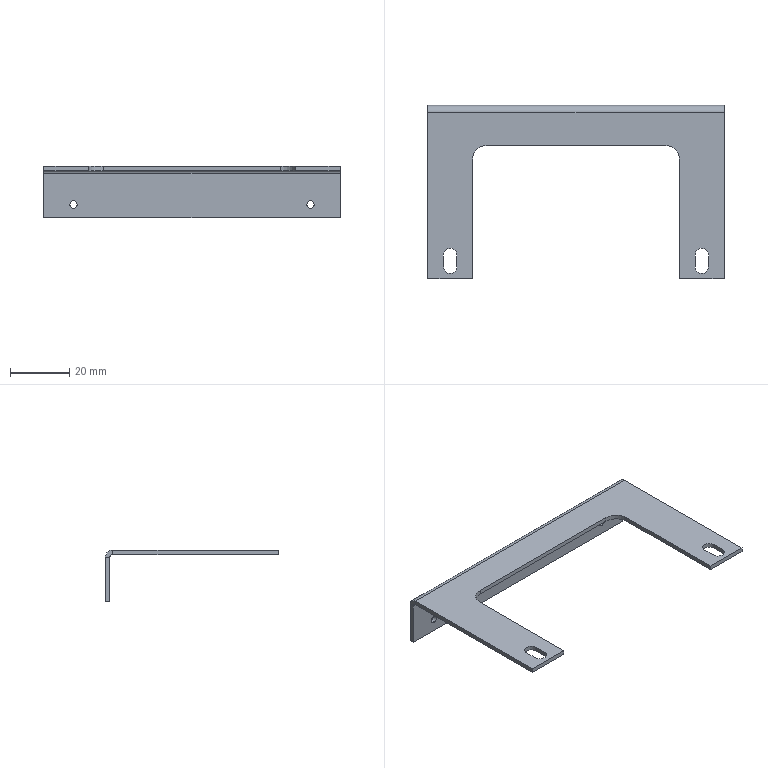Part | SolidWorks | features HoleWzd 2, Cut 1, FlatPattern 1, SMBaseFlange 1, SheetMetal 1 | 1 solid | 32 faces | box 100 x 58.5 x 17.5 mm | volume 6237 mm3 | plane 20 | cylinder 12 | commonest cylinder face diameters 2.5 x4 4.5 x4 10 x2 2 x1 5 x1
STEP:
#1=CARTESIAN_POINT('',(90.,58.5,-10.25));
#2=VERTEX_POINT('',#1);
#3=CARTESIAN_POINT('',(90.,58.5,-12.75));
#4=VERTEX_POINT('',#3);
#5=CARTESIAN_POINT('',(90.,58.5,-11.5));
#6=DIRECTION('',(0.,-1.,0.));
#7=DIRECTION('',(0.,0.,-1.));
#8=AXIS2_PLACEMENT_3D('',#5,#6,#7);
#9=CIRCLE('',#8,1.25);
#10=EDGE_CURVE('',#2,#4,#9,.T.);
#11=ORIENTED_EDGE('',*,*,#10,.F.);
#12=CARTESIAN_POINT('',(90.,57.,-10.25));
#13=VERTEX_POINT('',#12);
#14=CARTESIAN_POINT('',(90.,57.,-10.25));
#15=DIRECTION('',(0.,-1.,0.));
#16=VECTOR('',#15,1000.);
#17=LINE('',#14,#16);
#18=EDGE_CURVE('',#2,#13,#17,.T.);
#19=ORIENTED_EDGE('',*,*,#18,.T.);
#20=CARTESIAN_POINT('',(90.,57.,-12.75));
#21=VERTEX_POINT('',#20);
#22=CARTESIAN_POINT('',(90.,57.,-11.5));
#23=DIRECTION('',(0.,-1.,0.));
#24=DIRECTION('',(0.,0.,-1.));
#25=AXIS2_PLACEMENT_3D('',#22,#23,#24);
#26=CIRCLE('',#25,1.25);
#27=EDGE_CURVE('',#13,#21,#26,.T.);
#28=ORIENTED_EDGE('',*,*,#27,.T.);
#29=CARTESIAN_POINT('',(90.,57.,-12.75));
#30=DIRECTION('',(0.,-1.,0.));
#31=VECTOR('',#30,1000.);
#32=LINE('',#29,#31);
#33=EDGE_CURVE('',#4,#21,#32,.T.);
#34=ORIENTED_EDGE('',*,*,#33,.F.);
#35=EDGE_LOOP('',(#11,#19,#28,#34));
#36=FACE_OUTER_BOUND('',#35,.T.);
#37=CARTESIAN_POINT('',(90.,57.,-11.5));
#38=DIRECTION('',(0.,-1.,0.));
#39=DIRECTION('',(0.,0.,-1.));
#40=AXIS2_PLACEMENT_3D('',#37,#38,#39);
#41=CYLINDRICAL_SURFACE('',#40,1.25);
#42=ADVANCED_FACE('',(#36),#41,.F.);
#43=CARTESIAN_POINT('',(10.,58.5,-10.25));
#44=VERTEX_POINT('',#43);
#45=CARTESIAN_POINT('',(10.,58.5,-12.75));
#46=VERTEX_POINT('',#45);
#47=CARTESIAN_POINT('',(10.,58.5,-11.5));
#48=DIRECTION('',(0.,-1.,0.));
#49=DIRECTION('',(0.,0.,-1.));
#50=AXIS2_PLACEMENT_3D('',#47,#48,#49);
#51=CIRCLE('',#50,1.25);
#52=EDGE_CURVE('',#44,#46,#51,.T.);
#53=ORIENTED_EDGE('',*,*,#52,.F.);
#54=CARTESIAN_POINT('',(10.,57.,-10.25));
#55=VERTEX_POINT('',#54);
#56=CARTESIAN_POINT('',(10.,57.,-10.25));
#57=DIRECTION('',(0.,-1.,0.));
#58=VECTOR('',#57,1000.);
#59=LINE('',#56,#58);
#60=EDGE_CURVE('',#44,#55,#59,.T.);
#61=ORIENTED_EDGE('',*,*,#60,.T.);
#62=CARTESIAN_POINT('',(10.,57.,-12.75));
#63=VERTEX_POINT('',#62);
#64=CARTESIAN_POINT('',(10.,57.,-11.5));
#65=DIRECTION('',(0.,-1.,0.));
#66=DIRECTION('',(0.,0.,-1.));
#67=AXIS2_PLACEMENT_3D('',#64,#65,#66);
#68=CIRCLE('',#67,1.25);
#69=EDGE_CURVE('',#55,#63,#68,.T.);
#70=ORIENTED_EDGE('',*,*,#69,.T.);
#71=CARTESIAN_POINT('',(10.,57.,-12.75));
#72=DIRECTION('',(0.,-1.,0.));
#73=VECTOR('',#72,1000.);
#74=LINE('',#71,#73);
#75=EDGE_CURVE('',#46,#63,#74,.T.);
#76=ORIENTED_EDGE('',*,*,#75,.F.);
#77=EDGE_LOOP('',(#53,#61,#70,#76));
#78=FACE_OUTER_BOUND('',#77,.T.);
#79=CARTESIAN_POINT('',(10.,57.,-11.5));
#80=DIRECTION('',(0.,-1.,0.));
#81=DIRECTION('',(0.,0.,-1.));
#82=AXIS2_PLACEMENT_3D('',#79,#80,#81);
#83=CYLINDRICAL_SURFACE('',#82,1.25);
#84=ADVANCED_FACE('',(#78),#83,.F.);
#85=CARTESIAN_POINT('',(15.,0.,0.));
#86=VERTEX_POINT('',#85);
#87=CARTESIAN_POINT('',(15.,0.,1.5));
#88=VERTEX_POINT('',#87);
#89=CARTESIAN_POINT('',(15.,0.,-16.));
#90=DIRECTION('',(0.,0.,1.));
#91=VECTOR('',#90,1000.);
#92=LINE('',#89,#91);
#93=EDGE_CURVE('',#86,#88,#92,.T.);
#94=ORIENTED_EDGE('',*,*,#93,.T.);
#95=CARTESIAN_POINT('',(0.,0.,1.5));
#96=VERTEX_POINT('',#95);
#97=CARTESIAN_POINT('',(100.,0.,1.5));
#98=DIRECTION('',(-1.,0.,0.));
#99=VECTOR('',#98,1000.);
#100=LINE('',#97,#99);
#101=EDGE_CURVE('',#88,#96,#100,.T.);
#102=ORIENTED_EDGE('',*,*,#101,.T.);
#103=CARTESIAN_POINT('',(0.,0.,0.));
#104=VERTEX_POINT('',#103);
#105=CARTESIAN_POINT('',(0.,0.,0.));
#106=DIRECTION('',(0.,0.,1.));
#107=VECTOR('',#106,1000.);
#108=LINE('',#105,#107);
#109=EDGE_CURVE('',#104,#96,#108,.T.);
#110=ORIENTED_EDGE('',*,*,#109,.F.);
#111=CARTESIAN_POINT('',(100.,0.,0.));
#112=DIRECTION('',(-1.,0.,0.));
#113=VECTOR('',#112,1000.);
#114=LINE('',#111,#113);
#115=EDGE_CURVE('',#86,#104,#114,.T.);
#116=ORIENTED_EDGE('',*,*,#115,.F.);
#117=EDGE_LOOP('',(#94,#102,#110,#116));
#118=FACE_OUTER_BOUND('',#117,.T.);
#119=CARTESIAN_POINT('',(100.,0.,0.));
#120=DIRECTION('',(0.,-1.,0.));
#121=DIRECTION('',(0.,0.,-1.));
#122=AXIS2_PLACEMENT_3D('',#119,#120,#121);
#123=PLANE('',#122);
#124=ADVANCED_FACE('',(#118),#123,.T.);
#125=CARTESIAN_POINT('',(100.,56.,0.));
#126=VERTEX_POINT('',#125);
#127=CARTESIAN_POINT('',(100.,56.,1.5));
#128=VERTEX_POINT('',#127);
#129=CARTESIAN_POINT('',(100.,56.,0.));
#130=DIRECTION('',(0.,0.,1.));
#131=VECTOR('',#130,1000.);
#132=LINE('',#129,#131);
#133=EDGE_CURVE('',#126,#128,#132,.T.);
#134=ORIENTED_EDGE('',*,*,#133,.F.);
#135=CARTESIAN_POINT('',(100.,57.,-1.));
#136=VERTEX_POINT('',#135);
#137=CARTESIAN_POINT('',(100.,56.,-1.));
#138=DIRECTION('',(1.,0.,0.));
#139=DIRECTION('',(0.,0.,-1.));
#140=AXIS2_PLACEMENT_3D('',#137,#138,#139);
#141=CIRCLE('',#140,1.);
#142=EDGE_CURVE('',#136,#126,#141,.T.);
#143=ORIENTED_EDGE('',*,*,#142,.F.);
#144=CARTESIAN_POINT('',(100.,58.5,-1.));
#145=VERTEX_POINT('',#144);
#146=CARTESIAN_POINT('',(100.,58.5,-1.));
#147=DIRECTION('',(0.,-1.,0.));
#148=VECTOR('',#147,1000.);
#149=LINE('',#146,#148);
#150=EDGE_CURVE('',#145,#136,#149,.T.);
#151=ORIENTED_EDGE('',*,*,#150,.F.);
#152=CARTESIAN_POINT('',(100.,56.,-1.));
#153=DIRECTION('',(1.,0.,0.));
#154=DIRECTION('',(0.,0.,-1.));
#155=AXIS2_PLACEMENT_3D('',#152,#153,#154);
#156=CIRCLE('',#155,2.5);
#157=EDGE_CURVE('',#145,#128,#156,.T.);
#158=ORIENTED_EDGE('',*,*,#157,.T.);
#159=EDGE_LOOP('',(#134,#143,#151,#158));
#160=FACE_OUTER_BOUND('',#159,.T.);
#161=CARTESIAN_POINT('',(100.,56.,0.));
#162=DIRECTION('',(1.,0.,0.));
#163=DIRECTION('',(0.,0.,-1.));
#164=AXIS2_PLACEMENT_3D('',#161,#162,#163);
#165=PLANE('',#164);
#166=ADVANCED_FACE('',(#160),#165,.T.);
#167=CARTESIAN_POINT('',(100.,0.,0.));
#168=VERTEX_POINT('',#167);
#169=CARTESIAN_POINT('',(100.,0.,0.));
#170=DIRECTION('',(0.,-1.,0.));
#171=VECTOR('',#170,1000.);
#172=LINE('',#169,#171);
#173=EDGE_CURVE('',#126,#168,#172,.T.);
#174=ORIENTED_EDGE('',*,*,#173,.F.);
#175=ORIENTED_EDGE('',*,*,#133,.T.);
#176=CARTESIAN_POINT('',(100.,0.,1.5));
#177=VERTEX_POINT('',#176);
#178=CARTESIAN_POINT('',(100.,0.,1.5));
#179=DIRECTION('',(0.,-1.,0.));
#180=VECTOR('',#179,1000.);
#181=LINE('',#178,#180);
#182=EDGE_CURVE('',#128,#177,#181,.T.);
#183=ORIENTED_EDGE('',*,*,#182,.T.);
#184=CARTESIAN_POINT('',(100.,0.,0.));
#185=DIRECTION('',(0.,0.,1.));
#186=VECTOR('',#185,1000.);
#187=LINE('',#184,#186);
#188=EDGE_CURVE('',#168,#177,#187,.T.);
#189=ORIENTED_EDGE('',*,*,#188,.F.);
#190=EDGE_LOOP('',(#174,#175,#183,#189));
#191=FACE_OUTER_BOUND('',#190,.T.);
#192=CARTESIAN_POINT('',(100.,58.5,-1.));
#193=DIRECTION('',(1.,0.,0.));
#194=DIRECTION('',(0.,0.,-1.));
#195=AXIS2_PLACEMENT_3D('',#192,#193,#194);
#196=PLANE('',#195);
#197=ADVANCED_FACE('',(#191),#196,.T.);
#198=CARTESIAN_POINT('',(0.,57.,-1.));
#199=VERTEX_POINT('',#198);
#200=CARTESIAN_POINT('',(0.,58.5,-1.));
#201=VERTEX_POINT('',#200);
#202=CARTESIAN_POINT('',(0.,57.,-1.));
#203=DIRECTION('',(0.,1.,0.));
#204=VECTOR('',#203,1000.);
#205=LINE('',#202,#204);
#206=EDGE_CURVE('',#199,#201,#205,.T.);
#207=ORIENTED_EDGE('',*,*,#206,.F.);
#208=CARTESIAN_POINT('',(0.,56.,0.));
#209=VERTEX_POINT('',#208);
#210=CARTESIAN_POINT('',(0.,56.,-1.));
#211=DIRECTION('',(1.,0.,0.));
#212=DIRECTION('',(0.,0.,-1.));
#213=AXIS2_PLACEMENT_3D('',#210,#211,#212);
#214=CIRCLE('',#213,1.);
#215=EDGE_CURVE('',#199,#209,#214,.T.);
#216=ORIENTED_EDGE('',*,*,#215,.T.);
#217=CARTESIAN_POINT('',(0.,56.,1.5));
#218=VERTEX_POINT('',#217);
#219=CARTESIAN_POINT('',(0.,56.,1.5));
#220=DIRECTION('',(0.,0.,-1.));
#221=VECTOR('',#220,1000.);
#222=LINE('',#219,#221);
#223=EDGE_CURVE('',#218,#209,#222,.T.);
#224=ORIENTED_EDGE('',*,*,#223,.F.);
#225=CARTESIAN_POINT('',(0.,56.,-1.));
#226=DIRECTION('',(1.,0.,0.));
#227=DIRECTION('',(0.,0.,-1.));
#228=AXIS2_PLACEMENT_3D('',#225,#226,#227);
#229=CIRCLE('',#228,2.5);
#230=EDGE_CURVE('',#201,#218,#229,.T.);
#231=ORIENTED_EDGE('',*,*,#230,.F.);
#232=EDGE_LOOP('',(#207,#216,#224,#231));
#233=FACE_OUTER_BOUND('',#232,.T.);
#234=CARTESIAN_POINT('',(0.,57.,-1.));
#235=DIRECTION('',(-1.,0.,0.));
#236=DIRECTION('',(0.,0.,1.));
#237=AXIS2_PLACEMENT_3D('',#234,#235,#236);
#238=PLANE('',#237);
#239=ADVANCED_FACE('',(#233),#238,.T.);
#240=CARTESIAN_POINT('',(0.,57.,-16.));
#241=VERTEX_POINT('',#240);
#242=CARTESIAN_POINT('',(0.,57.,0.));
#243=DIRECTION('',(0.,0.,1.));
#244=VECTOR('',#243,1000.);
#245=LINE('',#242,#244);
#246=EDGE_CURVE('',#241,#199,#245,.T.);
#247=ORIENTED_EDGE('',*,*,#246,.T.);
#248=ORIENTED_EDGE('',*,*,#206,.T.);
#249=CARTESIAN_POINT('',(0.,58.5,-16.));
#250=VERTEX_POINT('',#249);
#251=CARTESIAN_POINT('',(0.,58.5,0.));
#252=DIRECTION('',(0.,0.,1.));
#253=VECTOR('',#252,1000.);
#254=LINE('',#251,#253);
#255=EDGE_CURVE('',#250,#201,#254,.T.);
#256=ORIENTED_EDGE('',*,*,#255,.F.);
#257=CARTESIAN_POINT('',(0.,58.5,-16.));
#258=DIRECTION('',(0.,-1.,0.));
#259=VECTOR('',#258,1000.);
#260=LINE('',#257,#259);
#261=EDGE_CURVE('',#250,#241,#260,.T.);
#262=ORIENTED_EDGE('',*,*,#261,.T.);
#263=EDGE_LOOP('',(#247,#248,#256,#262));
#264=FACE_OUTER_BOUND('',#263,.T.);
#265=CARTESIAN_POINT('',(0.,56.,1.5));
#266=DIRECTION('',(-1.,0.,0.));
#267=DIRECTION('',(0.,0.,1.));
#268=AXIS2_PLACEMENT_3D('',#265,#266,#267);
#269=PLANE('',#268);
#270=ADVANCED_FACE('',(#264),#269,.T.);
#271=CARTESIAN_POINT('',(94.75,8.,1.5));
#272=VERTEX_POINT('',#271);
#273=CARTESIAN_POINT('',(90.25,8.,1.5));
#274=VERTEX_POINT('',#273);
#275=CARTESIAN_POINT('',(92.5,8.,1.5));
#276=DIRECTION('',(0.,0.,1.));
#277=DIRECTION('',(1.,0.,0.));
#278=AXIS2_PLACEMENT_3D('',#275,#276,#277);
#279=CIRCLE('',#278,2.25);
#280=EDGE_CURVE('',#272,#274,#279,.T.);
#281=ORIENTED_EDGE('',*,*,#280,.F.);
#282=CARTESIAN_POINT('',(94.75,4.,1.5));
#283=VERTEX_POINT('',#282);
#284=CARTESIAN_POINT('',(94.75,4.,1.5));
#285=DIRECTION('',(0.,1.,0.));
#286=VECTOR('',#285,1000.);
#287=LINE('',#284,#286);
#288=EDGE_CURVE('',#283,#272,#287,.T.);
#289=ORIENTED_EDGE('',*,*,#288,.F.);
#290=CARTESIAN_POINT('',(90.25,4.,1.5));
#291=VERTEX_POINT('',#290);
#292=CARTESIAN_POINT('',(92.5,4.,1.5));
#293=DIRECTION('',(0.,0.,1.));
#294=DIRECTION('',(1.,0.,0.));
#295=AXIS2_PLACEMENT_3D('',#292,#293,#294);
#296=CIRCLE('',#295,2.25);
#297=EDGE_CURVE('',#291,#283,#296,.T.);
#298=ORIENTED_EDGE('',*,*,#297,.F.);
#299=CARTESIAN_POINT('',(90.25,4.,1.5));
#300=DIRECTION('',(0.,1.,0.));
#301=VECTOR('',#300,1000.);
#302=LINE('',#299,#301);
#303=EDGE_CURVE('',#291,#274,#302,.T.);
#304=ORIENTED_EDGE('',*,*,#303,.T.);
#305=EDGE_LOOP('',(#281,#289,#298,#304));
#306=FACE_BOUND('',#305,.T.);
#307=CARTESIAN_POINT('',(9.75,4.,1.5));
#308=VERTEX_POINT('',#307);
#309=CARTESIAN_POINT('',(9.75,8.,1.5));
#310=VERTEX_POINT('',#309);
#311=CARTESIAN_POINT('',(9.75,4.,1.5));
#312=DIRECTION('',(0.,1.,0.));
#313=VECTOR('',#312,1000.);
#314=LINE('',#311,#313);
#315=EDGE_CURVE('',#308,#310,#314,.T.);
#316=ORIENTED_EDGE('',*,*,#315,.F.);
#317=CARTESIAN_POINT('',(5.25,4.,1.5));
#318=VERTEX_POINT('',#317);
#319=CARTESIAN_POINT('',(7.5,4.,1.5));
#320=DIRECTION('',(0.,0.,1.));
#321=DIRECTION('',(1.,0.,0.));
#322=AXIS2_PLACEMENT_3D('',#319,#320,#321);
#323=CIRCLE('',#322,2.25);
#324=EDGE_CURVE('',#318,#308,#323,.T.);
#325=ORIENTED_EDGE('',*,*,#324,.F.);
#326=CARTESIAN_POINT('',(5.25,8.,1.5));
#327=VERTEX_POINT('',#326);
#328=CARTESIAN_POINT('',(5.25,4.,1.5));
#329=DIRECTION('',(0.,1.,0.));
#330=VECTOR('',#329,1000.);
#331=LINE('',#328,#330);
#332=EDGE_CURVE('',#318,#327,#331,.T.);
#333=ORIENTED_EDGE('',*,*,#332,.T.);
#334=CARTESIAN_POINT('',(7.5,8.,1.5));
#335=DIRECTION('',(0.,0.,1.));
#336=DIRECTION('',(1.,0.,0.));
#337=AXIS2_PLACEMENT_3D('',#334,#335,#336);
#338=CIRCLE('',#337,2.25);
#339=EDGE_CURVE('',#310,#327,#338,.T.);
#340=ORIENTED_EDGE('',*,*,#339,.F.);
#341=EDGE_LOOP('',(#316,#325,#333,#340));
#342=FACE_BOUND('',#341,.T.);
#343=ORIENTED_EDGE('',*,*,#101,.F.);
#344=CARTESIAN_POINT('',(15.,40.,1.5));
#345=VERTEX_POINT('',#344);
#346=CARTESIAN_POINT('',(15.,0.,1.5));
#347=DIRECTION('',(0.,-1.,0.));
#348=VECTOR('',#347,1000.);
#349=LINE('',#346,#348);
#350=EDGE_CURVE('',#345,#88,#349,.T.);
#351=ORIENTED_EDGE('',*,*,#350,.F.);
#352=CARTESIAN_POINT('',(20.,45.,1.5));
#353=VERTEX_POINT('',#352);
#354=CARTESIAN_POINT('',(20.,40.,1.5));
#355=DIRECTION('',(0.,0.,1.));
#356=DIRECTION('',(-1.,0.,0.));
#357=AXIS2_PLACEMENT_3D('',#354,#355,#356);
#358=CIRCLE('',#357,5.);
#359=EDGE_CURVE('',#353,#345,#358,.T.);
#360=ORIENTED_EDGE('',*,*,#359,.F.);
#361=CARTESIAN_POINT('',(80.,45.,1.5));
#362=VERTEX_POINT('',#361);
#363=CARTESIAN_POINT('',(20.,45.,1.5));
#364=DIRECTION('',(-1.,0.,0.));
#365=VECTOR('',#364,1000.);
#366=LINE('',#363,#365);
#367=EDGE_CURVE('',#362,#353,#366,.T.);
#368=ORIENTED_EDGE('',*,*,#367,.F.);
#369=CARTESIAN_POINT('',(85.,40.,1.5));
#370=VERTEX_POINT('',#369);
#371=CARTESIAN_POINT('',(80.,40.,1.5));
#372=DIRECTION('',(0.,0.,1.));
#373=DIRECTION('',(-1.,0.,0.));
#374=AXIS2_PLACEMENT_3D('',#371,#372,#373);
#375=CIRCLE('',#374,5.);
#376=EDGE_CURVE('',#370,#362,#375,.T.);
#377=ORIENTED_EDGE('',*,*,#376,.F.);
#378=CARTESIAN_POINT('',(85.,0.,1.5));
#379=VERTEX_POINT('',#378);
#380=CARTESIAN_POINT('',(85.,0.,1.5));
#381=DIRECTION('',(0.,1.,0.));
#382=VECTOR('',#381,1000.);
#383=LINE('',#380,#382);
#384=EDGE_CURVE('',#379,#370,#383,.T.);
#385=ORIENTED_EDGE('',*,*,#384,.F.);
#386=CARTESIAN_POINT('',(100.,0.,1.5));
#387=DIRECTION('',(-1.,0.,0.));
#388=VECTOR('',#387,1000.);
#389=LINE('',#386,#388);
#390=EDGE_CURVE('',#177,#379,#389,.T.);
#391=ORIENTED_EDGE('',*,*,#390,.F.);
#392=ORIENTED_EDGE('',*,*,#182,.F.);
#393=CARTESIAN_POINT('',(100.,56.,1.5));
#394=DIRECTION('',(-1.,0.,0.));
#395=VECTOR('',#394,1000.);
#396=LINE('',#393,#395);
#397=EDGE_CURVE('',#128,#218,#396,.T.);
#398=ORIENTED_EDGE('',*,*,#397,.T.);
#399=CARTESIAN_POINT('',(0.,0.,1.5));
#400=DIRECTION('',(0.,-1.,0.));
#401=VECTOR('',#400,1000.);
#402=LINE('',#399,#401);
#403=EDGE_CURVE('',#218,#96,#402,.T.);
#404=ORIENTED_EDGE('',*,*,#403,.T.);
#405=EDGE_LOOP('',(#343,#351,#360,#368,#377,#385,#391,#392,#398,#404));
#406=FACE_OUTER_BOUND('',#405,.T.);
#407=CARTESIAN_POINT('',(100.,0.,1.5));
#408=DIRECTION('',(0.,0.,-1.));
#409=DIRECTION('',(-1.,0.,0.));
#410=AXIS2_PLACEMENT_3D('',#407,#408,#409);
#411=PLANE('',#410);
#412=ADVANCED_FACE('',(#306,#342,#406),#411,.F.);
#413=CARTESIAN_POINT('',(85.,0.,0.));
#414=VERTEX_POINT('',#413);
#415=CARTESIAN_POINT('',(85.,0.,-16.));
#416=DIRECTION('',(0.,0.,1.));
#417=VECTOR('',#416,1000.);
#418=LINE('',#415,#417);
#419=EDGE_CURVE('',#414,#379,#418,.T.);
#420=ORIENTED_EDGE('',*,*,#419,.F.);
#421=CARTESIAN_POINT('',(100.,0.,0.));
#422=DIRECTION('',(-1.,0.,0.));
#423=VECTOR('',#422,1000.);
#424=LINE('',#421,#423);
#425=EDGE_CURVE('',#168,#414,#424,.T.);
#426=ORIENTED_EDGE('',*,*,#425,.F.);
#427=ORIENTED_EDGE('',*,*,#188,.T.);
#428=ORIENTED_EDGE('',*,*,#390,.T.);
#429=EDGE_LOOP('',(#420,#426,#427,#428));
#430=FACE_OUTER_BOUND('',#429,.T.);
#431=CARTESIAN_POINT('',(100.,0.,0.));
#432=DIRECTION('',(0.,-1.,0.));
#433=DIRECTION('',(0.,0.,-1.));
#434=AXIS2_PLACEMENT_3D('',#431,#432,#433);
#435=PLANE('',#434);
#436=ADVANCED_FACE('',(#430),#435,.T.);
#437=CARTESIAN_POINT('',(90.25,8.,0.));
#438=VERTEX_POINT('',#437);
#439=CARTESIAN_POINT('',(94.75,8.,0.));
#440=VERTEX_POINT('',#439);
#441=CARTESIAN_POINT('',(92.5,8.,0.));
#442=DIRECTION('',(0.,0.,-1.));
#443=DIRECTION('',(-1.,0.,0.));
#444=AXIS2_PLACEMENT_3D('',#441,#442,#443);
#445=CIRCLE('',#444,2.25);
#446=EDGE_CURVE('',#438,#440,#445,.T.);
#447=ORIENTED_EDGE('',*,*,#446,.F.);
#448=CARTESIAN_POINT('',(90.25,4.,0.));
#449=VERTEX_POINT('',#448);
#450=CARTESIAN_POINT('',(90.25,0.,0.));
#451=DIRECTION('',(0.,1.,0.));
#452=VECTOR('',#451,1000.);
#453=LINE('',#450,#452);
#454=EDGE_CURVE('',#449,#438,#453,.T.);
#455=ORIENTED_EDGE('',*,*,#454,.F.);
#456=CARTESIAN_POINT('',(94.75,4.,0.));
#457=VERTEX_POINT('',#456);
#458=CARTESIAN_POINT('',(92.5,4.,0.));
#459=DIRECTION('',(0.,0.,-1.));
#460=DIRECTION('',(-1.,0.,0.));
#461=AXIS2_PLACEMENT_3D('',#458,#459,#460);
#462=CIRCLE('',#461,2.25);
#463=EDGE_CURVE('',#457,#449,#462,.T.);
#464=ORIENTED_EDGE('',*,*,#463,.F.);
#465=CARTESIAN_POINT('',(94.75,0.,0.));
#466=DIRECTION('',(0.,-1.,0.));
#467=VECTOR('',#466,1000.);
#468=LINE('',#465,#467);
#469=EDGE_CURVE('',#440,#457,#468,.T.);
#470=ORIENTED_EDGE('',*,*,#469,.F.);
#471=EDGE_LOOP('',(#447,#455,#464,#470));
#472=FACE_BOUND('',#471,.T.);
#473=CARTESIAN_POINT('',(5.25,8.,0.));
#474=VERTEX_POINT('',#473);
#475=CARTESIAN_POINT('',(9.75,8.,0.));
#476=VERTEX_POINT('',#475);
#477=CARTESIAN_POINT('',(7.5,8.,0.));
#478=DIRECTION('',(0.,0.,-1.));
#479=DIRECTION('',(-1.,0.,0.));
#480=AXIS2_PLACEMENT_3D('',#477,#478,#479);
#481=CIRCLE('',#480,2.25);
#482=EDGE_CURVE('',#474,#476,#481,.T.);
#483=ORIENTED_EDGE('',*,*,#482,.F.);
#484=CARTESIAN_POINT('',(5.25,4.,0.));
#485=VERTEX_POINT('',#484);
#486=CARTESIAN_POINT('',(5.25,0.,0.));
#487=DIRECTION('',(0.,1.,0.));
#488=VECTOR('',#487,1000.);
#489=LINE('',#486,#488);
#490=EDGE_CURVE('',#485,#474,#489,.T.);
#491=ORIENTED_EDGE('',*,*,#490,.F.);
#492=CARTESIAN_POINT('',(9.75,4.,0.));
#493=VERTEX_POINT('',#492);
#494=CARTESIAN_POINT('',(7.5,4.,0.));
#495=DIRECTION('',(0.,0.,-1.));
#496=DIRECTION('',(-1.,0.,0.));
#497=AXIS2_PLACEMENT_3D('',#494,#495,#496);
#498=CIRCLE('',#497,2.25);
#499=EDGE_CURVE('',#493,#485,#498,.T.);
#500=ORIENTED_EDGE('',*,*,#499,.F.);
#501=CARTESIAN_POINT('',(9.75,0.,0.));
#502=DIRECTION('',(0.,-1.,0.));
#503=VECTOR('',#502,1000.);
#504=LINE('',#501,#503);
#505=EDGE_CURVE('',#476,#493,#504,.T.);
#506=ORIENTED_EDGE('',*,*,#505,.F.);
#507=EDGE_LOOP('',(#483,#491,#500,#506));
#508=FACE_BOUND('',#507,.T.);
#509=CARTESIAN_POINT('',(15.,40.,0.));
#510=VERTEX_POINT('',#509);
#511=CARTESIAN_POINT('',(15.,0.,0.));
#512=DIRECTION('',(0.,1.,0.));
#513=VECTOR('',#512,1000.);
#514=LINE('',#511,#513);
#515=EDGE_CURVE('',#86,#510,#514,.T.);
#516=ORIENTED_EDGE('',*,*,#515,.F.);
#517=ORIENTED_EDGE('',*,*,#115,.T.);
#518=CARTESIAN_POINT('',(0.,0.,0.));
#519=DIRECTION('',(0.,-1.,0.));
#520=VECTOR('',#519,1000.);
#521=LINE('',#518,#520);
#522=EDGE_CURVE('',#209,#104,#521,.T.);
#523=ORIENTED_EDGE('',*,*,#522,.F.);
#524=CARTESIAN_POINT('',(100.,56.,0.));
#525=DIRECTION('',(-1.,0.,0.));
#526=VECTOR('',#525,1000.);
#527=LINE('',#524,#526);
#528=EDGE_CURVE('',#126,#209,#527,.T.);
#529=ORIENTED_EDGE('',*,*,#528,.F.);
#530=ORIENTED_EDGE('',*,*,#173,.T.);
#531=ORIENTED_EDGE('',*,*,#425,.T.);
#532=CARTESIAN_POINT('',(85.,40.,0.));
#533=VERTEX_POINT('',#532);
#534=CARTESIAN_POINT('',(85.,0.,0.));
#535=DIRECTION('',(0.,-1.,0.));
#536=VECTOR('',#535,1000.);
#537=LINE('',#534,#536);
#538=EDGE_CURVE('',#533,#414,#537,.T.);
#539=ORIENTED_EDGE('',*,*,#538,.F.);
#540=CARTESIAN_POINT('',(80.,45.,0.));
#541=VERTEX_POINT('',#540);
#542=CARTESIAN_POINT('',(80.,40.,0.));
#543=DIRECTION('',(0.,0.,-1.));
#544=DIRECTION('',(-1.,0.,0.));
#545=AXIS2_PLACEMENT_3D('',#542,#543,#544);
#546=CIRCLE('',#545,5.);
#547=EDGE_CURVE('',#541,#533,#546,.T.);
#548=ORIENTED_EDGE('',*,*,#547,.F.);
#549=CARTESIAN_POINT('',(20.,45.,0.));
#550=VERTEX_POINT('',#549);
#551=CARTESIAN_POINT('',(100.,45.,0.));
#552=DIRECTION('',(1.,0.,0.));
#553=VECTOR('',#552,1000.);
#554=LINE('',#551,#553);
#555=EDGE_CURVE('',#550,#541,#554,.T.);
#556=ORIENTED_EDGE('',*,*,#555,.F.);
#557=CARTESIAN_POINT('',(20.,40.,0.));
#558=DIRECTION('',(0.,0.,-1.));
#559=DIRECTION('',(-1.,0.,0.));
#560=AXIS2_PLACEMENT_3D('',#557,#558,#559);
#561=CIRCLE('',#560,5.);
#562=EDGE_CURVE('',#510,#550,#561,.T.);
#563=ORIENTED_EDGE('',*,*,#562,.F.);
#564=EDGE_LOOP('',(#516,#517,#523,#529,#530,#531,#539,#548,#556,#563));
#565=FACE_OUTER_BOUND('',#564,.T.);
#566=CARTESIAN_POINT('',(100.,0.,0.));
#567=DIRECTION('',(0.,0.,-1.));
#568=DIRECTION('',(-1.,0.,0.));
#569=AXIS2_PLACEMENT_3D('',#566,#567,#568);
#570=PLANE('',#569);
#571=ADVANCED_FACE('',(#472,#508,#565),#570,.T.);
#572=ORIENTED_EDGE('',*,*,#215,.F.);
#573=CARTESIAN_POINT('',(100.,57.,-1.));
#574=DIRECTION('',(-1.,0.,0.));
#575=VECTOR('',#574,1000.);
#576=LINE('',#573,#575);
#577=EDGE_CURVE('',#136,#199,#576,.T.);
#578=ORIENTED_EDGE('',*,*,#577,.F.);
#579=ORIENTED_EDGE('',*,*,#142,.T.);
#580=ORIENTED_EDGE('',*,*,#528,.T.);
#581=EDGE_LOOP('',(#572,#578,#579,#580));
#582=FACE_OUTER_BOUND('',#581,.T.);
#583=CARTESIAN_POINT('',(100.,56.,-1.));
#584=DIRECTION('',(-1.,0.,0.));
#585=DIRECTION('',(0.,0.,1.));
#586=AXIS2_PLACEMENT_3D('',#583,#584,#585);
#587=CYLINDRICAL_SURFACE('',#586,1.);
#588=ADVANCED_FACE('',(#582),#587,.F.);
#589=CARTESIAN_POINT('',(90.,57.,-11.5));
#590=DIRECTION('',(0.,-1.,0.));
#591=DIRECTION('',(0.,0.,-1.));
#592=AXIS2_PLACEMENT_3D('',#589,#590,#591);
#593=CIRCLE('',#592,1.25);
#594=EDGE_CURVE('',#21,#13,#593,.T.);
#595=ORIENTED_EDGE('',*,*,#594,.F.);
#596=ORIENTED_EDGE('',*,*,#27,.F.);
#597=EDGE_LOOP('',(#595,#596));
#598=FACE_BOUND('',#597,.T.);
#599=CARTESIAN_POINT('',(10.,57.,-11.5));
#600=DIRECTION('',(0.,-1.,0.));
#601=DIRECTION('',(0.,0.,-1.));
#602=AXIS2_PLACEMENT_3D('',#599,#600,#601);
#603=CIRCLE('',#602,1.25);
#604=EDGE_CURVE('',#63,#55,#603,.T.);
#605=ORIENTED_EDGE('',*,*,#604,.F.);
#606=ORIENTED_EDGE('',*,*,#69,.F.);
#607=EDGE_LOOP('',(#605,#606));
#608=FACE_BOUND('',#607,.T.);
#609=ORIENTED_EDGE('',*,*,#246,.F.);
#610=CARTESIAN_POINT('',(100.,57.,-16.));
#611=VERTEX_POINT('',#610);
#612=CARTESIAN_POINT('',(100.,57.,-16.));
#613=DIRECTION('',(-1.,0.,0.));
#614=VECTOR('',#613,1000.);
#615=LINE('',#612,#614);
#616=EDGE_CURVE('',#611,#241,#615,.T.);
#617=ORIENTED_EDGE('',*,*,#616,.F.);
#618=CARTESIAN_POINT('',(100.,57.,0.));
#619=DIRECTION('',(0.,0.,1.));
#620=VECTOR('',#619,1000.);
#621=LINE('',#618,#620);
#622=EDGE_CURVE('',#611,#136,#621,.T.);
#623=ORIENTED_EDGE('',*,*,#622,.T.);
#624=ORIENTED_EDGE('',*,*,#577,.T.);
#625=EDGE_LOOP('',(#609,#617,#623,#624));
#626=FACE_OUTER_BOUND('',#625,.T.);
#627=CARTESIAN_POINT('',(100.,57.,0.));
#628=DIRECTION('',(0.,-1.,0.));
#629=DIRECTION('',(0.,0.,-1.));
#630=AXIS2_PLACEMENT_3D('',#627,#628,#629);
#631=PLANE('',#630);
#632=ADVANCED_FACE('',(#598,#608,#626),#631,.T.);
#633=ORIENTED_EDGE('',*,*,#261,.F.);
#634=CARTESIAN_POINT('',(100.,58.5,-16.));
#635=VERTEX_POINT('',#634);
#636=CARTESIAN_POINT('',(100.,58.5,-16.));
#637=DIRECTION('',(-1.,0.,0.));
#638=VECTOR('',#637,1000.);
#639=LINE('',#636,#638);
#640=EDGE_CURVE('',#635,#250,#639,.T.);
#641=ORIENTED_EDGE('',*,*,#640,.F.);
#642=CARTESIAN_POINT('',(100.,58.5,-16.));
#643=DIRECTION('',(0.,-1.,0.));
#644=VECTOR('',#643,1000.);
#645=LINE('',#642,#644);
#646=EDGE_CURVE('',#635,#611,#645,.T.);
#647=ORIENTED_EDGE('',*,*,#646,.T.);
#648=ORIENTED_EDGE('',*,*,#616,.T.);
#649=EDGE_LOOP('',(#633,#641,#647,#648));
#650=FACE_OUTER_BOUND('',#649,.T.);
#651=CARTESIAN_POINT('',(100.,58.5,-16.));
#652=DIRECTION('',(0.,0.,-1.));
#653=DIRECTION('',(-1.,0.,0.));
#654=AXIS2_PLACEMENT_3D('',#651,#652,#653);
#655=PLANE('',#654);
#656=ADVANCED_FACE('',(#650),#655,.T.);
#657=CARTESIAN_POINT('',(90.,58.5,-11.5));
#658=DIRECTION('',(0.,-1.,0.));
#659=DIRECTION('',(0.,0.,-1.));
#660=AXIS2_PLACEMENT_3D('',#657,#658,#659);
#661=CIRCLE('',#660,1.25);
#662=EDGE_CURVE('',#4,#2,#661,.T.);
#663=ORIENTED_EDGE('',*,*,#662,.T.);
#664=ORIENTED_EDGE('',*,*,#10,.T.);
#665=EDGE_LOOP('',(#663,#664));
#666=FACE_BOUND('',#665,.T.);
#667=CARTESIAN_POINT('',(10.,58.5,-11.5));
#668=DIRECTION('',(0.,-1.,0.));
#669=DIRECTION('',(0.,0.,-1.));
#670=AXIS2_PLACEMENT_3D('',#667,#668,#669);
#671=CIRCLE('',#670,1.25);
#672=EDGE_CURVE('',#46,#44,#671,.T.);
#673=ORIENTED_EDGE('',*,*,#672,.T.);
#674=ORIENTED_EDGE('',*,*,#52,.T.);
#675=EDGE_LOOP('',(#673,#674));
#676=FACE_BOUND('',#675,.T.);
#677=ORIENTED_EDGE('',*,*,#255,.T.);
#678=CARTESIAN_POINT('',(100.,58.5,-1.));
#679=DIRECTION('',(-1.,0.,0.));
#680=VECTOR('',#679,1000.);
#681=LINE('',#678,#680);
#682=EDGE_CURVE('',#145,#201,#681,.T.);
#683=ORIENTED_EDGE('',*,*,#682,.F.);
#684=CARTESIAN_POINT('',(100.,58.5,0.));
#685=DIRECTION('',(0.,0.,1.));
#686=VECTOR('',#685,1000.);
#687=LINE('',#684,#686);
#688=EDGE_CURVE('',#635,#145,#687,.T.);
#689=ORIENTED_EDGE('',*,*,#688,.F.);
#690=ORIENTED_EDGE('',*,*,#640,.T.);
#691=EDGE_LOOP('',(#677,#683,#689,#690));
#692=FACE_OUTER_BOUND('',#691,.T.);
#693=CARTESIAN_POINT('',(100.,58.5,0.));
#694=DIRECTION('',(0.,-1.,0.));
#695=DIRECTION('',(0.,0.,-1.));
#696=AXIS2_PLACEMENT_3D('',#693,#694,#695);
#697=PLANE('',#696);
#698=ADVANCED_FACE('',(#666,#676,#692),#697,.F.);
#699=ORIENTED_EDGE('',*,*,#230,.T.);
#700=ORIENTED_EDGE('',*,*,#397,.F.);
#701=ORIENTED_EDGE('',*,*,#157,.F.);
#702=ORIENTED_EDGE('',*,*,#682,.T.);
#703=EDGE_LOOP('',(#699,#700,#701,#702));
#704=FACE_OUTER_BOUND('',#703,.T.);
#705=CARTESIAN_POINT('',(100.,56.,-1.));
#706=DIRECTION('',(-1.,0.,0.));
#707=DIRECTION('',(0.,0.,1.));
#708=AXIS2_PLACEMENT_3D('',#705,#706,#707);
#709=CYLINDRICAL_SURFACE('',#708,2.5);
#710=ADVANCED_FACE('',(#704),#709,.T.);
#711=ORIENTED_EDGE('',*,*,#688,.T.);
#712=ORIENTED_EDGE('',*,*,#150,.T.);
#713=ORIENTED_EDGE('',*,*,#622,.F.);
#714=ORIENTED_EDGE('',*,*,#646,.F.);
#715=EDGE_LOOP('',(#711,#712,#713,#714));
#716=FACE_OUTER_BOUND('',#715,.T.);
#717=CARTESIAN_POINT('',(100.,56.,-1.));
#718=DIRECTION('',(1.,0.,0.));
#719=DIRECTION('',(0.,0.,-1.));
#720=AXIS2_PLACEMENT_3D('',#717,#718,#719);
#721=PLANE('',#720);
#722=ADVANCED_FACE('',(#716),#721,.T.);
#723=ORIENTED_EDGE('',*,*,#403,.F.);
#724=ORIENTED_EDGE('',*,*,#223,.T.);
#725=ORIENTED_EDGE('',*,*,#522,.T.);
#726=ORIENTED_EDGE('',*,*,#109,.T.);
#727=EDGE_LOOP('',(#723,#724,#725,#726));
#728=FACE_OUTER_BOUND('',#727,.T.);
#729=CARTESIAN_POINT('',(0.,56.,-1.));
#730=DIRECTION('',(1.,0.,0.));
#731=DIRECTION('',(0.,0.,-1.));
#732=AXIS2_PLACEMENT_3D('',#729,#730,#731);
#733=PLANE('',#732);
#734=ADVANCED_FACE('',(#728),#733,.F.);
#735=ORIENTED_EDGE('',*,*,#515,.T.);
#736=CARTESIAN_POINT('',(15.,40.,-16.));
#737=DIRECTION('',(0.,0.,1.));
#738=VECTOR('',#737,1000.);
#739=LINE('',#736,#738);
#740=EDGE_CURVE('',#510,#345,#739,.T.);
#741=ORIENTED_EDGE('',*,*,#740,.T.);
#742=ORIENTED_EDGE('',*,*,#350,.T.);
#743=ORIENTED_EDGE('',*,*,#93,.F.);
#744=EDGE_LOOP('',(#735,#741,#742,#743));
#745=FACE_OUTER_BOUND('',#744,.T.);
#746=CARTESIAN_POINT('',(15.,0.,-16.));
#747=DIRECTION('',(-1.,0.,0.));
#748=DIRECTION('',(0.,0.,1.));
#749=AXIS2_PLACEMENT_3D('',#746,#747,#748);
#750=PLANE('',#749);
#751=ADVANCED_FACE('',(#745),#750,.F.);
#752=ORIENTED_EDGE('',*,*,#562,.T.);
#753=CARTESIAN_POINT('',(20.,45.,-16.));
#754=DIRECTION('',(0.,0.,1.));
#755=VECTOR('',#754,1000.);
#756=LINE('',#753,#755);
#757=EDGE_CURVE('',#550,#353,#756,.T.);
#758=ORIENTED_EDGE('',*,*,#757,.T.);
#759=ORIENTED_EDGE('',*,*,#359,.T.);
#760=ORIENTED_EDGE('',*,*,#740,.F.);
#761=EDGE_LOOP('',(#752,#758,#759,#760));
#762=FACE_OUTER_BOUND('',#761,.T.);
#763=CARTESIAN_POINT('',(20.,40.,-16.));
#764=DIRECTION('',(0.,0.,1.));
#765=DIRECTION('',(1.,0.,0.));
#766=AXIS2_PLACEMENT_3D('',#763,#764,#765);
#767=CYLINDRICAL_SURFACE('',#766,5.);
#768=ADVANCED_FACE('',(#762),#767,.F.);
#769=ORIENTED_EDGE('',*,*,#555,.T.);
#770=CARTESIAN_POINT('',(80.,45.,-16.));
#771=DIRECTION('',(0.,0.,1.));
#772=VECTOR('',#771,1000.);
#773=LINE('',#770,#772);
#774=EDGE_CURVE('',#541,#362,#773,.T.);
#775=ORIENTED_EDGE('',*,*,#774,.T.);
#776=ORIENTED_EDGE('',*,*,#367,.T.);
#777=ORIENTED_EDGE('',*,*,#757,.F.);
#778=EDGE_LOOP('',(#769,#775,#776,#777));
#779=FACE_OUTER_BOUND('',#778,.T.);
#780=CARTESIAN_POINT('',(20.,45.,-16.));
#781=DIRECTION('',(0.,1.,0.));
#782=DIRECTION('',(0.,0.,1.));
#783=AXIS2_PLACEMENT_3D('',#780,#781,#782);
#784=PLANE('',#783);
#785=ADVANCED_FACE('',(#779),#784,.F.);
#786=ORIENTED_EDGE('',*,*,#547,.T.);
#787=CARTESIAN_POINT('',(85.,40.,-16.));
#788=DIRECTION('',(0.,0.,1.));
#789=VECTOR('',#788,1000.);
#790=LINE('',#787,#789);
#791=EDGE_CURVE('',#533,#370,#790,.T.);
#792=ORIENTED_EDGE('',*,*,#791,.T.);
#793=ORIENTED_EDGE('',*,*,#376,.T.);
#794=ORIENTED_EDGE('',*,*,#774,.F.);
#795=EDGE_LOOP('',(#786,#792,#793,#794));
#796=FACE_OUTER_BOUND('',#795,.T.);
#797=CARTESIAN_POINT('',(80.,40.,-16.));
#798=DIRECTION('',(0.,0.,1.));
#799=DIRECTION('',(1.,0.,0.));
#800=AXIS2_PLACEMENT_3D('',#797,#798,#799);
#801=CYLINDRICAL_SURFACE('',#800,5.);
#802=ADVANCED_FACE('',(#796),#801,.F.);
#803=ORIENTED_EDGE('',*,*,#538,.T.);
#804=ORIENTED_EDGE('',*,*,#419,.T.);
#805=ORIENTED_EDGE('',*,*,#384,.T.);
#806=ORIENTED_EDGE('',*,*,#791,.F.);
#807=EDGE_LOOP('',(#803,#804,#805,#806));
#808=FACE_OUTER_BOUND('',#807,.T.);
#809=CARTESIAN_POINT('',(85.,0.,-16.));
#810=DIRECTION('',(1.,0.,0.));
#811=DIRECTION('',(0.,0.,-1.));
#812=AXIS2_PLACEMENT_3D('',#809,#810,#811);
#813=PLANE('',#812);
#814=ADVANCED_FACE('',(#808),#813,.F.);
#815=ORIENTED_EDGE('',*,*,#482,.T.);
#816=CARTESIAN_POINT('',(9.75,8.,-8.6));
#817=DIRECTION('',(0.,0.,-1.));
#818=VECTOR('',#817,1000.);
#819=LINE('',#816,#818);
#820=EDGE_CURVE('',#310,#476,#819,.T.);
#821=ORIENTED_EDGE('',*,*,#820,.F.);
#822=ORIENTED_EDGE('',*,*,#339,.T.);
#823=CARTESIAN_POINT('',(5.25,8.,1.5));
#824=DIRECTION('',(0.,0.,1.));
#825=VECTOR('',#824,1000.);
#826=LINE('',#823,#825);
#827=EDGE_CURVE('',#474,#327,#826,.T.);
#828=ORIENTED_EDGE('',*,*,#827,.F.);
#829=EDGE_LOOP('',(#815,#821,#822,#828));
#830=FACE_OUTER_BOUND('',#829,.T.);
#831=CARTESIAN_POINT('',(7.5,8.,1.5));
#832=DIRECTION('',(0.,0.,1.));
#833=DIRECTION('',(1.,0.,0.));
#834=AXIS2_PLACEMENT_3D('',#831,#832,#833);
#835=CYLINDRICAL_SURFACE('',#834,2.25);
#836=ADVANCED_FACE('',(#830),#835,.F.);
#837=ORIENTED_EDGE('',*,*,#499,.T.);
#838=CARTESIAN_POINT('',(5.25,4.,1.5));
#839=DIRECTION('',(0.,0.,-1.));
#840=VECTOR('',#839,1000.);
#841=LINE('',#838,#840);
#842=EDGE_CURVE('',#318,#485,#841,.T.);
#843=ORIENTED_EDGE('',*,*,#842,.F.);
#844=ORIENTED_EDGE('',*,*,#324,.T.);
#845=CARTESIAN_POINT('',(9.75,4.,-8.6));
#846=DIRECTION('',(0.,0.,-1.));
#847=VECTOR('',#846,1000.);
#848=LINE('',#845,#847);
#849=EDGE_CURVE('',#308,#493,#848,.T.);
#850=ORIENTED_EDGE('',*,*,#849,.T.);
#851=EDGE_LOOP('',(#837,#843,#844,#850));
#852=FACE_OUTER_BOUND('',#851,.T.);
#853=CARTESIAN_POINT('',(7.5,4.,1.5));
#854=DIRECTION('',(0.,0.,1.));
#855=DIRECTION('',(1.,0.,0.));
#856=AXIS2_PLACEMENT_3D('',#853,#854,#855);
#857=CYLINDRICAL_SURFACE('',#856,2.25);
#858=ADVANCED_FACE('',(#852),#857,.F.);
#859=ORIENTED_EDGE('',*,*,#490,.T.);
#860=ORIENTED_EDGE('',*,*,#827,.T.);
#861=ORIENTED_EDGE('',*,*,#332,.F.);
#862=ORIENTED_EDGE('',*,*,#842,.T.);
#863=EDGE_LOOP('',(#859,#860,#861,#862));
#864=FACE_OUTER_BOUND('',#863,.T.);
#865=CARTESIAN_POINT('',(5.25,4.,1.5));
#866=DIRECTION('',(-1.,0.,0.));
#867=DIRECTION('',(0.,0.,1.));
#868=AXIS2_PLACEMENT_3D('',#865,#866,#867);
#869=PLANE('',#868);
#870=ADVANCED_FACE('',(#864),#869,.F.);
#871=ORIENTED_EDGE('',*,*,#505,.T.);
#872=ORIENTED_EDGE('',*,*,#849,.F.);
#873=ORIENTED_EDGE('',*,*,#315,.T.);
#874=ORIENTED_EDGE('',*,*,#820,.T.);
#875=EDGE_LOOP('',(#871,#872,#873,#874));
#876=FACE_OUTER_BOUND('',#875,.T.);
#877=CARTESIAN_POINT('',(9.75,4.,-8.6));
#878=DIRECTION('',(1.,0.,0.));
#879=DIRECTION('',(0.,0.,-1.));
#880=AXIS2_PLACEMENT_3D('',#877,#878,#879);
#881=PLANE('',#880);
#882=ADVANCED_FACE('',(#876),#881,.F.);
#883=ORIENTED_EDGE('',*,*,#446,.T.);
#884=CARTESIAN_POINT('',(94.75,8.,-8.6));
#885=DIRECTION('',(0.,0.,-1.));
#886=VECTOR('',#885,1000.);
#887=LINE('',#884,#886);
#888=EDGE_CURVE('',#272,#440,#887,.T.);
#889=ORIENTED_EDGE('',*,*,#888,.F.);
#890=ORIENTED_EDGE('',*,*,#280,.T.);
#891=CARTESIAN_POINT('',(90.25,8.,1.5));
#892=DIRECTION('',(0.,0.,1.));
#893=VECTOR('',#892,1000.);
#894=LINE('',#891,#893);
#895=EDGE_CURVE('',#438,#274,#894,.T.);
#896=ORIENTED_EDGE('',*,*,#895,.F.);
#897=EDGE_LOOP('',(#883,#889,#890,#896));
#898=FACE_OUTER_BOUND('',#897,.T.);
#899=CARTESIAN_POINT('',(92.5,8.,1.5));
#900=DIRECTION('',(0.,0.,1.));
#901=DIRECTION('',(1.,0.,0.));
#902=AXIS2_PLACEMENT_3D('',#899,#900,#901);
#903=CYLINDRICAL_SURFACE('',#902,2.25);
#904=ADVANCED_FACE('',(#898),#903,.F.);
#905=ORIENTED_EDGE('',*,*,#463,.T.);
#906=CARTESIAN_POINT('',(90.25,4.,1.5));
#907=DIRECTION('',(0.,0.,-1.));
#908=VECTOR('',#907,1000.);
#909=LINE('',#906,#908);
#910=EDGE_CURVE('',#291,#449,#909,.T.);
#911=ORIENTED_EDGE('',*,*,#910,.F.);
#912=ORIENTED_EDGE('',*,*,#297,.T.);
#913=CARTESIAN_POINT('',(94.75,4.,-8.6));
#914=DIRECTION('',(0.,0.,-1.));
#915=VECTOR('',#914,1000.);
#916=LINE('',#913,#915);
#917=EDGE_CURVE('',#283,#457,#916,.T.);
#918=ORIENTED_EDGE('',*,*,#917,.T.);
#919=EDGE_LOOP('',(#905,#911,#912,#918));
#920=FACE_OUTER_BOUND('',#919,.T.);
#921=CARTESIAN_POINT('',(92.5,4.,1.5));
#922=DIRECTION('',(0.,0.,1.));
#923=DIRECTION('',(1.,0.,0.));
#924=AXIS2_PLACEMENT_3D('',#921,#922,#923);
#925=CYLINDRICAL_SURFACE('',#924,2.25);
#926=ADVANCED_FACE('',(#920),#925,.F.);
#927=ORIENTED_EDGE('',*,*,#454,.T.);
#928=ORIENTED_EDGE('',*,*,#895,.T.);
#929=ORIENTED_EDGE('',*,*,#303,.F.);
#930=ORIENTED_EDGE('',*,*,#910,.T.);
#931=EDGE_LOOP('',(#927,#928,#929,#930));
#932=FACE_OUTER_BOUND('',#931,.T.);
#933=CARTESIAN_POINT('',(90.25,4.,1.5));
#934=DIRECTION('',(-1.,0.,0.));
#935=DIRECTION('',(0.,0.,1.));
#936=AXIS2_PLACEMENT_3D('',#933,#934,#935);
#937=PLANE('',#936);
#938=ADVANCED_FACE('',(#932),#937,.F.);
#939=ORIENTED_EDGE('',*,*,#469,.T.);
#940=ORIENTED_EDGE('',*,*,#917,.F.);
#941=ORIENTED_EDGE('',*,*,#288,.T.);
#942=ORIENTED_EDGE('',*,*,#888,.T.);
#943=EDGE_LOOP('',(#939,#940,#941,#942));
#944=FACE_OUTER_BOUND('',#943,.T.);
#945=CARTESIAN_POINT('',(94.75,4.,-8.6));
#946=DIRECTION('',(1.,0.,0.));
#947=DIRECTION('',(0.,0.,-1.));
#948=AXIS2_PLACEMENT_3D('',#945,#946,#947);
#949=PLANE('',#948);
#950=ADVANCED_FACE('',(#944),#949,.F.);
#951=ORIENTED_EDGE('',*,*,#60,.F.);
#952=ORIENTED_EDGE('',*,*,#672,.F.);
#953=ORIENTED_EDGE('',*,*,#75,.T.);
#954=ORIENTED_EDGE('',*,*,#604,.T.);
#955=EDGE_LOOP('',(#951,#952,#953,#954));
#956=FACE_OUTER_BOUND('',#955,.T.);
#957=CARTESIAN_POINT('',(10.,57.,-11.5));
#958=DIRECTION('',(0.,-1.,0.));
#959=DIRECTION('',(0.,0.,-1.));
#960=AXIS2_PLACEMENT_3D('',#957,#958,#959);
#961=CYLINDRICAL_SURFACE('',#960,1.25);
#962=ADVANCED_FACE('',(#956),#961,.F.);
#963=ORIENTED_EDGE('',*,*,#18,.F.);
#964=ORIENTED_EDGE('',*,*,#662,.F.);
#965=ORIENTED_EDGE('',*,*,#33,.T.);
#966=ORIENTED_EDGE('',*,*,#594,.T.);
#967=EDGE_LOOP('',(#963,#964,#965,#966));
#968=FACE_OUTER_BOUND('',#967,.T.);
#969=CARTESIAN_POINT('',(90.,57.,-11.5));
#970=DIRECTION('',(0.,-1.,0.));
#971=DIRECTION('',(0.,0.,-1.));
#972=AXIS2_PLACEMENT_3D('',#969,#970,#971);
#973=CYLINDRICAL_SURFACE('',#972,1.25);
#974=ADVANCED_FACE('',(#968),#973,.F.);
#975=CLOSED_SHELL('',(#42,#84,#124,#166,#197,#239,#270,#412,#436,#571,#588,#632,#656,#698,#710,#722,#734,#751,#768,#785,#802,#814,#836,#858,#870,#882,#904,#926,#938,#950,#962,#974));
#976=MANIFOLD_SOLID_BREP('',#975);
#977=CARTESIAN_POINT('',(0.,0.,0.));
#978=DIRECTION('',(0.,0.,1.));
#979=DIRECTION('',(1.,0.,0.));
#980=AXIS2_PLACEMENT_3D('',#977,#978,#979);
#981=(LENGTH_UNIT()NAMED_UNIT(*)SI_UNIT(.MILLI.,.METRE.));
#982=UNCERTAINTY_MEASURE_WITH_UNIT(LENGTH_MEASURE(0.00001),#981,'','');
#983=(NAMED_UNIT(*)PLANE_ANGLE_UNIT()SI_UNIT($,.RADIAN.));
#984=(NAMED_UNIT(*)SI_UNIT($,.STERADIAN.)SOLID_ANGLE_UNIT());
#985=(GEOMETRIC_REPRESENTATION_CONTEXT(3)GLOBAL_UNCERTAINTY_ASSIGNED_CONTEXT((#982))GLOBAL_UNIT_ASSIGNED_CONTEXT((#981,#983,#984))REPRESENTATION_CONTEXT('',''));
#986=ADVANCED_BREP_SHAPE_REPRESENTATION('',(#976,#980),#985);